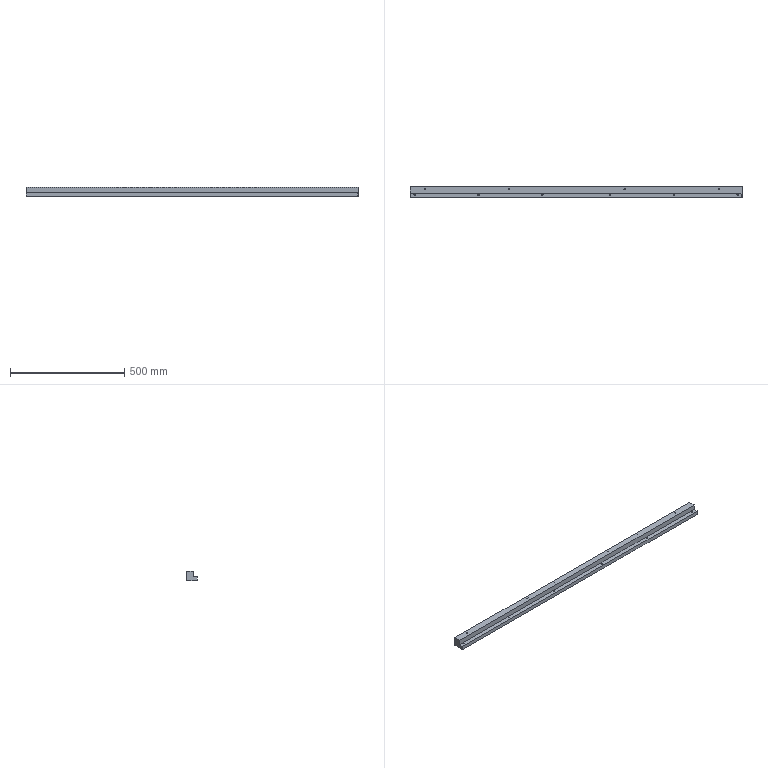Part | STEP file | J013-EBZ05-04-06 | 1 solid | 262 faces | box 1454 x 48 x 40 mm | volume 2132315 mm3 | cylinder 148 | cone 68 | plane 46 | commonest cylinder face diameters 6 x44 5.1 x32 4.2 x24 5 x24 8.6 x8 10 x8